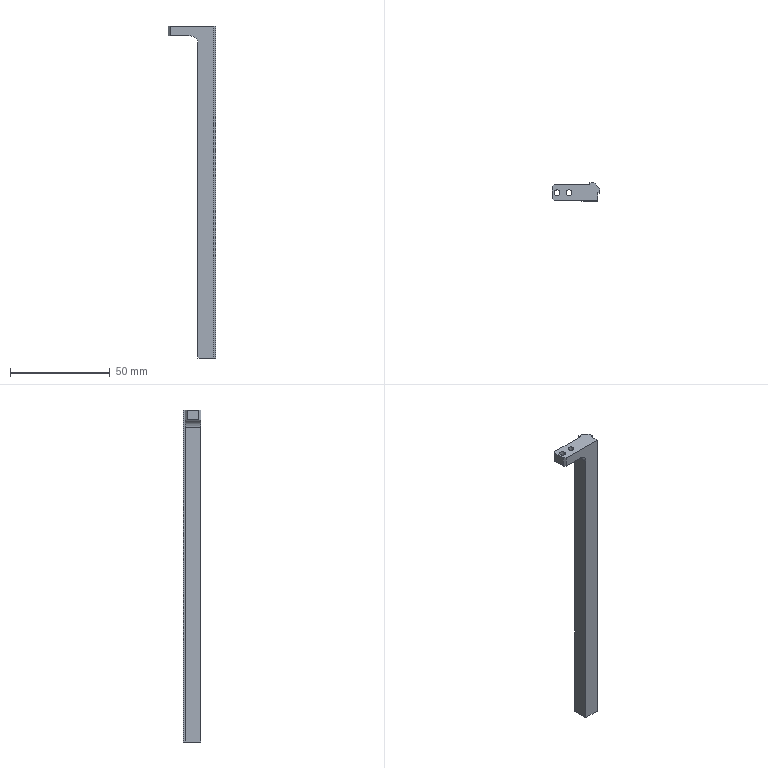CAM job | NX | 3+2 milling, drilling | part box 24 x 9 x 166.5 mm | stock box 28.5 x 10 x 176 mm
Tools:
number,name,description,diameter,corner_radius,flute_length,length,flutes
0,D8-25-D8-60-3T-ROUGH,D8-25-D8-60-3T-粗,8.0,0.0,25.0,60.0,2
0,D8-25-D8-60-3T-FINISH,D8-25-D8-60-3T,8.0,0.0,25.0,60.0,3
0,FACEMILL_D63,D63面刀,63.0,0.0,30.0,30.0,4
0,DRILL_D2.3-29-55,钻刀D2.1-29-55,2.3,0.0,29.0,55.0,2
0,FORMTAP_M2.5-12-D3-39,挤压M2.5-12-D3-39,2.5,0.0,13.0,15.0,2
0,D8R0-FINISH,Milling Tool-5 Parameters,8.0,0.0,50.0,75.0,2
0,DJ-D3,Countersink,3.0,0.0,0.0,60.0,2
0,DJ-D8,Countersink,8.0,0.0,0.0,60.0,2
0,DRILL_D2.9-39-67,钻刀D2.8-39-67,2.9,0.0,39.0,67.0,2
0,D50,Milling Tool-5 Parameters,50.0,0.0,50.0,75.0,2
0,D1.8_DRILL,Drilling Tool,1.8,0.0,35.0,50.0,2
0,M2,Drilling Tool,2.0,0.0,35.0,50.0,4
Operations:
program,operation,operation_type,tool,method,geometry_group,spindle_rpm,surface_speed,feed_per_tooth,feed_cut,feed_plunge,cut_length_mm,path_length_mm,cut_time_min,machine_time_min
A-G54,FACE_MILLING,FaceMilling,FACEMILL_D63,METHOD,WORKPIECE,4000.0,791.0,0.05,800.0,100.0,252.9,292.9,0.3161,0.3221
A-G54,DYNAMIC_ROUGH,CavityMilling,D8-25-D8-60-3T-ROUGH,METHOD,WORKPIECE,6500.0,100.0,0.1178,3000.0,100.0,3504.353,3747.725,1.159,1.184
A-G54,PLANAR_MILL_COPY_1_COPY_COPY,PlanarMilling,D8R0-FINISH,METHOD,WORKPIECE,6500.0,163.0,0.0385,500.0,100.0,817.33,879.33,1.688,1.697
A-G54,PLANAR_MILL_2,PlanarMilling,DJ-D3,METHOD,WORKPIECE,3500.0,32.0,0.1429,1000.0,100.0,395.76,433.76,0.3958,0.3996
A-G54,PLANAR_MILL_2_COPY,PlanarMilling,DJ-D3,METHOD,WORKPIECE,3500.0,32.0,0.0857,600.0,100.0,17.4,55.8,0.029,0.0328
A-G54,PLANAR_MILL_2_COPY_COPY,PlanarMilling,DJ-D3,METHOD,WORKPIECE,3500.0,32.0,0.0857,600.0,100.0,17.4,55.8,0.029,0.0328
D01,DRILLING_2,Operation,DJ-D8,METHOD,D-G55,2000.0,50.0,0.05,200.0,0.0,9.0,67.708,0.045,0.0509
D02,DRILLING_2_COPY,Operation,DRILL_D2.9-39-67,METHOD,D-G55,2500.0,22.0,0.04,200.0,0.0,20.0,89.708,0.1,0.107
B-G56,DRILLING_3,Operation,DJ-D3,METHOD,B-G56,2000.0,50.0,0.05,200.0,0.0,8.0,64.418,0.04,0.0456
B-G56,DRILLING_3_COPY,Operation,D1.8_DRILL,METHOD,B-G56,2000.0,50.0,0.05,200.0,0.0,22.0,92.418,0.11,0.117
B-G56,DRILLING_3_COPY_COPY,Operation,M2,METHOD,B-G56,300.0,1.0,0.1,120.0,0.0,19.0,86.418,0.1583,0.1651
B01,FACE_MILLING_COPY,FaceMilling,D50,METHOD,D-G57,4000.0,628.0,0.1875,1500.0,100.0,1389.0,2727.45,0.926,1.069
B01,FACE_MILLING_COPY_COPY,FaceMilling,D50,METHOD,D-G57,4000.0,628.0,0.1,800.0,100.0,231.5,283.5,0.2894,0.2972
B01,PLANAR_MILL,PlanarMilling,D50,METHOD,D-G57,4000.0,628.0,0.075,600.0,100.0,272.5,308.3,0.4542,0.4577
B02,PLANAR_MILL_COPY_2,PlanarMilling,D8-25-D8-60-3T-FINISH,METHOD,D-G57,5500.0,207.0,0.1364,1500.0,100.0,51.0,146.329,0.034,0.0465
B02,PLANAR_MILL_COPY_2_COPY,PlanarMilling,D8-25-D8-60-3T-FINISH,METHOD,D-G57,5500.0,207.0,0.1364,1500.0,100.0,178.5,220.3,0.119,0.1253
B02,PLANAR_MILL_COPY_2_COPY_COPY,PlanarMilling,D8-25-D8-60-3T-FINISH,METHOD,D-G57,5500.0,138.0,0.0485,800.0,100.0,178.5,220.5,0.2231,0.2294
B04,DRILLING,Operation,DJ-D3,METHOD,D-G57,2000.0,18.0,0.05,200.0,0.0,4.2,165.482,0.021,0.0371
B04,PLANAR_MILL_COPY_2_COPY_1_COPY_1,PlanarMilling,DJ-D3,METHOD,D-G57,5000.0,125.0,0.1,1000.0,100.0,350.47,391.67,0.3505,0.3566
B04,PLANAR_MILL_COPY_2_COPY_1_COPY_1_COPY,PlanarMilling,DJ-D3,METHOD,D-G57,5000.0,125.0,0.1,1000.0,100.0,203.589,243.589,0.2036,0.2095
B04,PLANAR_MILL_COPY_2_COPY_1_COPY_1_COPY_COPY,PlanarMilling,DJ-D3,METHOD,D-G57,5000.0,47.0,0.06,600.0,100.0,13.8,52.2,0.023,0.0288
B04,PLANAR_MILL_COPY_2_COPY_1_COPY_1_COPY_COPY_COPY,PlanarMilling,DJ-D3,METHOD,D-G57,5000.0,47.0,0.06,600.0,100.0,13.8,52.2,0.023,0.0288
B05,DRILLING_COPY,Operation,D1.8_DRILL,METHOD,D-G57,2000.0,11.0,0.025,100.0,0.0,15.0,187.082,0.15,0.1672
B06,DRILLING_COPY_COPY,Operation,M2,METHOD,D-G57,400.0,2.0,0.1,160.0,0.0,12.0,181.082,0.075,0.0919
G58,PLANAR_MILL_3,PlanarMilling,DJ-D3,METHOD,G58,4500.0,42.0,0.0889,800.0,100.0,33.2,115.0,0.0415,0.0497
G58,DRILLING_1,Operation,DJ-D3,METHOD,G58,2500.0,23.0,0.04,200.0,0.0,4.1,78.2,0.0205,0.0279
G58,DRILLING_1_COPY,Operation,DRILL_D2.3-29-55,METHOD,G58,2500.0,23.0,0.04,200.0,0.0,10.0,90.0,0.05,0.058
G58,DRILLING_1_COPY_COPY,Operation,FORMTAP_M2.5-12-D3-39,METHOD,G58,300.0,2.0,0.225,135.0,0.0,9.0,88.0,0.0667,0.0746
C01,PLANAR_MILL_COPY_2_COPY_1_COPY_1_COPY_1,PlanarMilling,D8-25-D8-60-3T-ROUGH,METHOD,C-G59,5000.0,125.0,0.12,1200.0,100.0,178.5,220.3,0.1488,0.155
C01,ZLEVEL_PROFILE,ZLevelMilling,D8-25-D8-60-3T-ROUGH,METHOD,C-G59,5000.0,125.0,0.3,3000.0,100.0,884.5,930.329,0.2948,0.3015
C01,PLANAR_MILL_COPY_2_COPY_1_COPY_1_COPY_1_COPY_2,PlanarMilling,D8R0-FINISH,METHOD,C-G59,5000.0,125.0,0.12,1200.0,100.0,178.5,220.5,0.1488,0.1551
C02,PLANAR_MILL_COPY_2_COPY_1_COPY_1_COPY_1_COPY_COPY,PlanarMilling,DJ-D8,METHOD,C-G59,5000.0,125.0,0.08,800.0,100.0,179.5,226.5,0.2244,0.2314
C03,DRILLING_COPY_1,Operation,DJ-D3,METHOD,C-G59,2000.0,18.0,0.05,200.0,0.0,6.3,275.778,0.0315,0.0584
C03,PLANAR_MILL_COPY_2_COPY_1_COPY_1_COPY_1_COPY_COPY_COPY,PlanarMilling,DJ-D3,METHOD,C-G59,5000.0,47.0,0.1,1000.0,100.0,178.113,219.713,0.1781,0.1844
C03,PLANAR_MILL_COPY_2_COPY_1_COPY_1_COPY_1_COPY_COPY_COPY_COPY,PlanarMilling,DJ-D3,METHOD,C-G59,5000.0,47.0,0.1,1000.0,100.0,172.0,216.0,0.172,0.1786
C04,DRILLING_COPY_COPY_1,Operation,D1.8_DRILL,METHOD,C-G59,2000.0,11.0,0.025,100.0,0.0,22.5,308.178,0.225,0.2536
C05,DRILLING_COPY_COPY_COPY,Operation,M2,METHOD,C-G59,300.0,1.0,0.1333,160.0,0.0,18.0,299.178,0.1125,0.1406